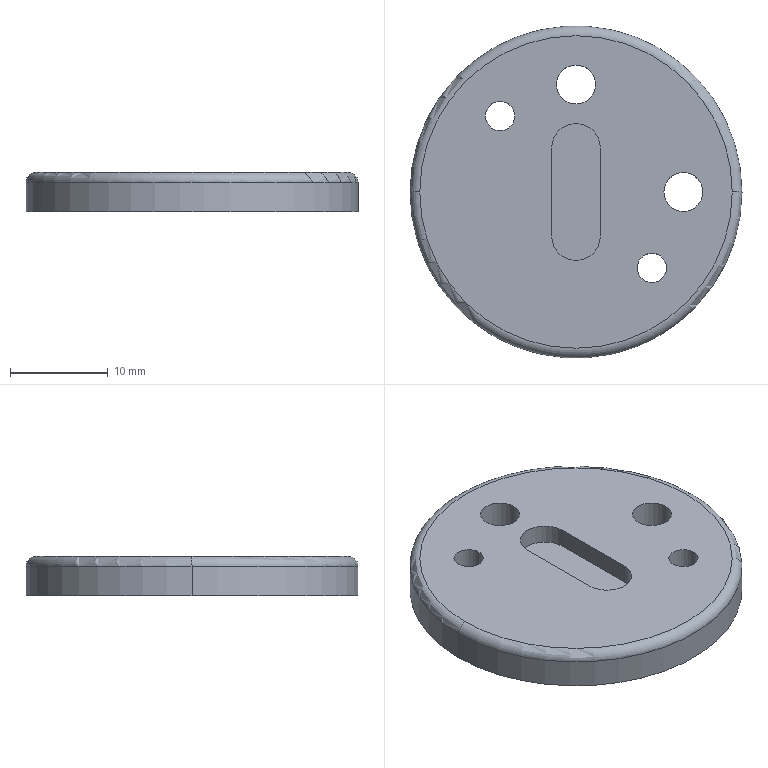Part | SolidWorks | features ICE 2, Extrusion 1, Fillet 1 | 1 solid | 19 faces | box 34 x 34 x 4 mm | volume 3323 mm3 | cylinder 12 | plane 5 | torus 2 | commonest cylinder face diameters 3 x4 4 x4 5 x2 34 x2
STEP:
#1=CARTESIAN_POINT('',(-17.,0.,3.));
#2=VERTEX_POINT('',#1);
#3=CARTESIAN_POINT('',(17.,0.,3.));
#4=VERTEX_POINT('',#3);
#5=CARTESIAN_POINT('',(0.,0.,3.));
#6=DIRECTION('',(0.,0.,-1.));
#7=DIRECTION('',(1.,0.,0.));
#8=AXIS2_PLACEMENT_3D('',#5,#6,#7);
#9=CIRCLE('',#8,17.);
#10=EDGE_CURVE('',#2,#4,#9,.T.);
#11=ORIENTED_EDGE('',*,*,#10,.F.);
#12=CARTESIAN_POINT('',(-16.,0.,4.));
#13=VERTEX_POINT('',#12);
#14=CARTESIAN_POINT('',(-16.,0.,3.));
#15=DIRECTION('',(0.,1.,0.));
#16=DIRECTION('',(-1.,0.,0.));
#17=AXIS2_PLACEMENT_3D('',#14,#15,#16);
#18=CIRCLE('',#17,1.);
#19=EDGE_CURVE('',#2,#13,#18,.T.);
#20=ORIENTED_EDGE('',*,*,#19,.T.);
#21=CARTESIAN_POINT('',(16.,0.,4.));
#22=VERTEX_POINT('',#21);
#23=CARTESIAN_POINT('',(0.,0.,4.));
#24=DIRECTION('',(0.,0.,1.));
#25=DIRECTION('',(1.,0.,0.));
#26=AXIS2_PLACEMENT_3D('',#23,#24,#25);
#27=CIRCLE('',#26,16.);
#28=EDGE_CURVE('',#22,#13,#27,.T.);
#29=ORIENTED_EDGE('',*,*,#28,.F.);
#30=CARTESIAN_POINT('',(16.,0.,3.));
#31=DIRECTION('',(0.,-1.,0.));
#32=DIRECTION('',(0.,0.,-1.));
#33=AXIS2_PLACEMENT_3D('',#30,#31,#32);
#34=CIRCLE('',#33,1.);
#35=EDGE_CURVE('',#4,#22,#34,.T.);
#36=ORIENTED_EDGE('',*,*,#35,.F.);
#37=EDGE_LOOP('',(#11,#20,#29,#36));
#38=FACE_OUTER_BOUND('',#37,.T.);
#39=CARTESIAN_POINT('',(0.,0.,3.));
#40=DIRECTION('',(0.,0.,1.));
#41=DIRECTION('',(1.,0.,0.));
#42=AXIS2_PLACEMENT_3D('',#39,#40,#41);
#43=TOROIDAL_SURFACE('',#42,16.,1.);
#44=ADVANCED_FACE('',(#38),#43,.T.);
#45=CARTESIAN_POINT('',(6.278,-7.778,0.));
#46=VERTEX_POINT('',#45);
#47=CARTESIAN_POINT('',(9.278,-7.778,0.));
#48=VERTEX_POINT('',#47);
#49=CARTESIAN_POINT('',(7.778,-7.778,0.));
#50=DIRECTION('',(0.,0.,1.));
#51=DIRECTION('',(1.,0.,0.));
#52=AXIS2_PLACEMENT_3D('',#49,#50,#51);
#53=CIRCLE('',#52,1.5);
#54=EDGE_CURVE('',#46,#48,#53,.T.);
#55=ORIENTED_EDGE('',*,*,#54,.F.);
#56=CARTESIAN_POINT('',(6.278,-7.778,4.));
#57=VERTEX_POINT('',#56);
#58=CARTESIAN_POINT('',(6.278,-7.778,0.));
#59=DIRECTION('',(0.,0.,1.));
#60=VECTOR('',#59,1000.);
#61=LINE('',#58,#60);
#62=EDGE_CURVE('',#46,#57,#61,.T.);
#63=ORIENTED_EDGE('',*,*,#62,.T.);
#64=CARTESIAN_POINT('',(9.278,-7.778,4.));
#65=VERTEX_POINT('',#64);
#66=CARTESIAN_POINT('',(7.778,-7.778,4.));
#67=DIRECTION('',(0.,0.,1.));
#68=DIRECTION('',(1.,0.,0.));
#69=AXIS2_PLACEMENT_3D('',#66,#67,#68);
#70=CIRCLE('',#69,1.5);
#71=EDGE_CURVE('',#57,#65,#70,.T.);
#72=ORIENTED_EDGE('',*,*,#71,.T.);
#73=CARTESIAN_POINT('',(9.278,-7.778,0.));
#74=DIRECTION('',(0.,0.,1.));
#75=VECTOR('',#74,1000.);
#76=LINE('',#73,#75);
#77=EDGE_CURVE('',#48,#65,#76,.T.);
#78=ORIENTED_EDGE('',*,*,#77,.F.);
#79=EDGE_LOOP('',(#55,#63,#72,#78));
#80=FACE_OUTER_BOUND('',#79,.T.);
#81=CARTESIAN_POINT('',(7.778,-7.778,0.));
#82=DIRECTION('',(0.,0.,1.));
#83=DIRECTION('',(1.,0.,0.));
#84=AXIS2_PLACEMENT_3D('',#81,#82,#83);
#85=CYLINDRICAL_SURFACE('',#84,1.5);
#86=ADVANCED_FACE('',(#80),#85,.F.);
#87=CARTESIAN_POINT('',(-9.278,7.778,0.));
#88=VERTEX_POINT('',#87);
#89=CARTESIAN_POINT('',(-6.278,7.778,0.));
#90=VERTEX_POINT('',#89);
#91=CARTESIAN_POINT('',(-7.778,7.778,0.));
#92=DIRECTION('',(0.,0.,1.));
#93=DIRECTION('',(1.,0.,0.));
#94=AXIS2_PLACEMENT_3D('',#91,#92,#93);
#95=CIRCLE('',#94,1.5);
#96=EDGE_CURVE('',#88,#90,#95,.T.);
#97=ORIENTED_EDGE('',*,*,#96,.F.);
#98=CARTESIAN_POINT('',(-9.278,7.778,4.));
#99=VERTEX_POINT('',#98);
#100=CARTESIAN_POINT('',(-9.278,7.778,0.));
#101=DIRECTION('',(0.,0.,1.));
#102=VECTOR('',#101,1000.);
#103=LINE('',#100,#102);
#104=EDGE_CURVE('',#88,#99,#103,.T.);
#105=ORIENTED_EDGE('',*,*,#104,.T.);
#106=CARTESIAN_POINT('',(-6.278,7.778,4.));
#107=VERTEX_POINT('',#106);
#108=CARTESIAN_POINT('',(-7.778,7.778,4.));
#109=DIRECTION('',(0.,0.,1.));
#110=DIRECTION('',(1.,0.,0.));
#111=AXIS2_PLACEMENT_3D('',#108,#109,#110);
#112=CIRCLE('',#111,1.5);
#113=EDGE_CURVE('',#99,#107,#112,.T.);
#114=ORIENTED_EDGE('',*,*,#113,.T.);
#115=CARTESIAN_POINT('',(-6.278,7.778,0.));
#116=DIRECTION('',(0.,0.,1.));
#117=VECTOR('',#116,1000.);
#118=LINE('',#115,#117);
#119=EDGE_CURVE('',#90,#107,#118,.T.);
#120=ORIENTED_EDGE('',*,*,#119,.F.);
#121=EDGE_LOOP('',(#97,#105,#114,#120));
#122=FACE_OUTER_BOUND('',#121,.T.);
#123=CARTESIAN_POINT('',(-7.778,7.778,0.));
#124=DIRECTION('',(0.,0.,1.));
#125=DIRECTION('',(1.,0.,0.));
#126=AXIS2_PLACEMENT_3D('',#123,#124,#125);
#127=CYLINDRICAL_SURFACE('',#126,1.5);
#128=ADVANCED_FACE('',(#122),#127,.F.);
#129=CARTESIAN_POINT('',(9.,0.,0.));
#130=VERTEX_POINT('',#129);
#131=CARTESIAN_POINT('',(13.,0.,0.));
#132=VERTEX_POINT('',#131);
#133=CARTESIAN_POINT('',(11.,0.,0.));
#134=DIRECTION('',(0.,0.,1.));
#135=DIRECTION('',(1.,0.,0.));
#136=AXIS2_PLACEMENT_3D('',#133,#134,#135);
#137=CIRCLE('',#136,2.);
#138=EDGE_CURVE('',#130,#132,#137,.T.);
#139=ORIENTED_EDGE('',*,*,#138,.F.);
#140=CARTESIAN_POINT('',(9.,0.,4.));
#141=VERTEX_POINT('',#140);
#142=CARTESIAN_POINT('',(9.,0.,0.));
#143=DIRECTION('',(0.,0.,1.));
#144=VECTOR('',#143,1000.);
#145=LINE('',#142,#144);
#146=EDGE_CURVE('',#130,#141,#145,.T.);
#147=ORIENTED_EDGE('',*,*,#146,.T.);
#148=CARTESIAN_POINT('',(13.,0.,4.));
#149=VERTEX_POINT('',#148);
#150=CARTESIAN_POINT('',(11.,0.,4.));
#151=DIRECTION('',(0.,0.,1.));
#152=DIRECTION('',(1.,0.,0.));
#153=AXIS2_PLACEMENT_3D('',#150,#151,#152);
#154=CIRCLE('',#153,2.);
#155=EDGE_CURVE('',#141,#149,#154,.T.);
#156=ORIENTED_EDGE('',*,*,#155,.T.);
#157=CARTESIAN_POINT('',(13.,0.,0.));
#158=DIRECTION('',(0.,0.,1.));
#159=VECTOR('',#158,1000.);
#160=LINE('',#157,#159);
#161=EDGE_CURVE('',#132,#149,#160,.T.);
#162=ORIENTED_EDGE('',*,*,#161,.F.);
#163=EDGE_LOOP('',(#139,#147,#156,#162));
#164=FACE_OUTER_BOUND('',#163,.T.);
#165=CARTESIAN_POINT('',(11.,0.,0.));
#166=DIRECTION('',(0.,0.,1.));
#167=DIRECTION('',(1.,0.,0.));
#168=AXIS2_PLACEMENT_3D('',#165,#166,#167);
#169=CYLINDRICAL_SURFACE('',#168,2.);
#170=ADVANCED_FACE('',(#164),#169,.F.);
#171=CARTESIAN_POINT('',(-2.,11.,0.));
#172=VERTEX_POINT('',#171);
#173=CARTESIAN_POINT('',(2.,11.,0.));
#174=VERTEX_POINT('',#173);
#175=CARTESIAN_POINT('',(0.,11.,0.));
#176=DIRECTION('',(0.,0.,1.));
#177=DIRECTION('',(1.,0.,0.));
#178=AXIS2_PLACEMENT_3D('',#175,#176,#177);
#179=CIRCLE('',#178,2.);
#180=EDGE_CURVE('',#172,#174,#179,.T.);
#181=ORIENTED_EDGE('',*,*,#180,.F.);
#182=CARTESIAN_POINT('',(-2.,11.,4.));
#183=VERTEX_POINT('',#182);
#184=CARTESIAN_POINT('',(-2.,11.,0.));
#185=DIRECTION('',(0.,0.,1.));
#186=VECTOR('',#185,1000.);
#187=LINE('',#184,#186);
#188=EDGE_CURVE('',#172,#183,#187,.T.);
#189=ORIENTED_EDGE('',*,*,#188,.T.);
#190=CARTESIAN_POINT('',(2.,11.,4.));
#191=VERTEX_POINT('',#190);
#192=CARTESIAN_POINT('',(0.,11.,4.));
#193=DIRECTION('',(0.,0.,1.));
#194=DIRECTION('',(1.,0.,0.));
#195=AXIS2_PLACEMENT_3D('',#192,#193,#194);
#196=CIRCLE('',#195,2.);
#197=EDGE_CURVE('',#183,#191,#196,.T.);
#198=ORIENTED_EDGE('',*,*,#197,.T.);
#199=CARTESIAN_POINT('',(2.,11.,0.));
#200=DIRECTION('',(0.,0.,1.));
#201=VECTOR('',#200,1000.);
#202=LINE('',#199,#201);
#203=EDGE_CURVE('',#174,#191,#202,.T.);
#204=ORIENTED_EDGE('',*,*,#203,.F.);
#205=EDGE_LOOP('',(#181,#189,#198,#204));
#206=FACE_OUTER_BOUND('',#205,.T.);
#207=CARTESIAN_POINT('',(0.,11.,0.));
#208=DIRECTION('',(0.,0.,1.));
#209=DIRECTION('',(1.,0.,0.));
#210=AXIS2_PLACEMENT_3D('',#207,#208,#209);
#211=CYLINDRICAL_SURFACE('',#210,2.);
#212=ADVANCED_FACE('',(#206),#211,.F.);
#213=ORIENTED_EDGE('',*,*,#10,.T.);
#214=CARTESIAN_POINT('',(17.,0.,0.));
#215=VERTEX_POINT('',#214);
#216=CARTESIAN_POINT('',(17.,0.,4.));
#217=DIRECTION('',(0.,0.,-1.));
#218=VECTOR('',#217,1000.);
#219=LINE('',#216,#218);
#220=EDGE_CURVE('',#4,#215,#219,.T.);
#221=ORIENTED_EDGE('',*,*,#220,.T.);
#222=CARTESIAN_POINT('',(-17.,0.,0.));
#223=VERTEX_POINT('',#222);
#224=CARTESIAN_POINT('',(0.,0.,0.));
#225=DIRECTION('',(0.,0.,1.));
#226=DIRECTION('',(1.,0.,0.));
#227=AXIS2_PLACEMENT_3D('',#224,#225,#226);
#228=CIRCLE('',#227,17.);
#229=EDGE_CURVE('',#215,#223,#228,.T.);
#230=ORIENTED_EDGE('',*,*,#229,.T.);
#231=CARTESIAN_POINT('',(-17.,0.,4.));
#232=DIRECTION('',(0.,0.,-1.));
#233=VECTOR('',#232,1000.);
#234=LINE('',#231,#233);
#235=EDGE_CURVE('',#2,#223,#234,.T.);
#236=ORIENTED_EDGE('',*,*,#235,.F.);
#237=EDGE_LOOP('',(#213,#221,#230,#236));
#238=FACE_OUTER_BOUND('',#237,.T.);
#239=CARTESIAN_POINT('',(0.,0.,4.));
#240=DIRECTION('',(0.,0.,-1.));
#241=DIRECTION('',(-1.,0.,0.));
#242=AXIS2_PLACEMENT_3D('',#239,#240,#241);
#243=CYLINDRICAL_SURFACE('',#242,17.);
#244=ADVANCED_FACE('',(#238),#243,.T.);
#245=ORIENTED_EDGE('',*,*,#220,.F.);
#246=CARTESIAN_POINT('',(0.,0.,3.));
#247=DIRECTION('',(0.,0.,-1.));
#248=DIRECTION('',(1.,0.,0.));
#249=AXIS2_PLACEMENT_3D('',#246,#247,#248);
#250=CIRCLE('',#249,17.);
#251=EDGE_CURVE('',#4,#2,#250,.T.);
#252=ORIENTED_EDGE('',*,*,#251,.T.);
#253=ORIENTED_EDGE('',*,*,#235,.T.);
#254=CARTESIAN_POINT('',(0.,0.,0.));
#255=DIRECTION('',(0.,0.,1.));
#256=DIRECTION('',(1.,0.,0.));
#257=AXIS2_PLACEMENT_3D('',#254,#255,#256);
#258=CIRCLE('',#257,17.);
#259=EDGE_CURVE('',#223,#215,#258,.T.);
#260=ORIENTED_EDGE('',*,*,#259,.T.);
#261=EDGE_LOOP('',(#245,#252,#253,#260));
#262=FACE_OUTER_BOUND('',#261,.T.);
#263=CARTESIAN_POINT('',(0.,0.,4.));
#264=DIRECTION('',(0.,0.,-1.));
#265=DIRECTION('',(-1.,0.,0.));
#266=AXIS2_PLACEMENT_3D('',#263,#264,#265);
#267=CYLINDRICAL_SURFACE('',#266,17.);
#268=ADVANCED_FACE('',(#262),#267,.T.);
#269=ORIENTED_EDGE('',*,*,#28,.T.);
#270=CARTESIAN_POINT('',(0.,0.,4.));
#271=DIRECTION('',(0.,0.,1.));
#272=DIRECTION('',(1.,0.,0.));
#273=AXIS2_PLACEMENT_3D('',#270,#271,#272);
#274=CIRCLE('',#273,16.);
#275=EDGE_CURVE('',#13,#22,#274,.T.);
#276=ORIENTED_EDGE('',*,*,#275,.T.);
#277=EDGE_LOOP('',(#269,#276));
#278=FACE_OUTER_BOUND('',#277,.T.);
#279=CARTESIAN_POINT('',(7.778,-7.778,4.));
#280=DIRECTION('',(0.,0.,1.));
#281=DIRECTION('',(1.,0.,0.));
#282=AXIS2_PLACEMENT_3D('',#279,#280,#281);
#283=CIRCLE('',#282,1.5);
#284=EDGE_CURVE('',#65,#57,#283,.T.);
#285=ORIENTED_EDGE('',*,*,#284,.F.);
#286=ORIENTED_EDGE('',*,*,#71,.F.);
#287=EDGE_LOOP('',(#285,#286));
#288=FACE_BOUND('',#287,.T.);
#289=CARTESIAN_POINT('',(-7.778,7.778,4.));
#290=DIRECTION('',(0.,0.,1.));
#291=DIRECTION('',(1.,0.,0.));
#292=AXIS2_PLACEMENT_3D('',#289,#290,#291);
#293=CIRCLE('',#292,1.5);
#294=EDGE_CURVE('',#107,#99,#293,.T.);
#295=ORIENTED_EDGE('',*,*,#294,.F.);
#296=ORIENTED_EDGE('',*,*,#113,.F.);
#297=EDGE_LOOP('',(#295,#296));
#298=FACE_BOUND('',#297,.T.);
#299=CARTESIAN_POINT('',(11.,0.,4.));
#300=DIRECTION('',(0.,0.,1.));
#301=DIRECTION('',(1.,0.,0.));
#302=AXIS2_PLACEMENT_3D('',#299,#300,#301);
#303=CIRCLE('',#302,2.);
#304=EDGE_CURVE('',#149,#141,#303,.T.);
#305=ORIENTED_EDGE('',*,*,#304,.F.);
#306=ORIENTED_EDGE('',*,*,#155,.F.);
#307=EDGE_LOOP('',(#305,#306));
#308=FACE_BOUND('',#307,.T.);
#309=CARTESIAN_POINT('',(0.,11.,4.));
#310=DIRECTION('',(0.,0.,1.));
#311=DIRECTION('',(1.,0.,0.));
#312=AXIS2_PLACEMENT_3D('',#309,#310,#311);
#313=CIRCLE('',#312,2.);
#314=EDGE_CURVE('',#191,#183,#313,.T.);
#315=ORIENTED_EDGE('',*,*,#314,.F.);
#316=ORIENTED_EDGE('',*,*,#197,.F.);
#317=EDGE_LOOP('',(#315,#316));
#318=FACE_BOUND('',#317,.T.);
#319=CARTESIAN_POINT('',(2.5,4.5,4.));
#320=VERTEX_POINT('',#319);
#321=CARTESIAN_POINT('',(-2.5,4.5,4.));
#322=VERTEX_POINT('',#321);
#323=CARTESIAN_POINT('',(0.,4.5,4.));
#324=DIRECTION('',(0.,0.,1.));
#325=DIRECTION('',(1.,0.,0.));
#326=AXIS2_PLACEMENT_3D('',#323,#324,#325);
#327=CIRCLE('',#326,2.5);
#328=EDGE_CURVE('',#320,#322,#327,.T.);
#329=ORIENTED_EDGE('',*,*,#328,.F.);
#330=CARTESIAN_POINT('',(2.5,-4.5,4.));
#331=VERTEX_POINT('',#330);
#332=CARTESIAN_POINT('',(2.5,4.5,4.));
#333=DIRECTION('',(0.,1.,0.));
#334=VECTOR('',#333,1000.);
#335=LINE('',#332,#334);
#336=EDGE_CURVE('',#331,#320,#335,.T.);
#337=ORIENTED_EDGE('',*,*,#336,.F.);
#338=CARTESIAN_POINT('',(-2.5,-4.5,4.));
#339=VERTEX_POINT('',#338);
#340=CARTESIAN_POINT('',(0.,-4.5,4.));
#341=DIRECTION('',(0.,0.,1.));
#342=DIRECTION('',(1.,0.,0.));
#343=AXIS2_PLACEMENT_3D('',#340,#341,#342);
#344=CIRCLE('',#343,2.5);
#345=EDGE_CURVE('',#339,#331,#344,.T.);
#346=ORIENTED_EDGE('',*,*,#345,.F.);
#347=CARTESIAN_POINT('',(-2.5,4.5,4.));
#348=DIRECTION('',(0.,-1.,0.));
#349=VECTOR('',#348,1000.);
#350=LINE('',#347,#349);
#351=EDGE_CURVE('',#322,#339,#350,.T.);
#352=ORIENTED_EDGE('',*,*,#351,.F.);
#353=EDGE_LOOP('',(#329,#337,#346,#352));
#354=FACE_BOUND('',#353,.T.);
#355=CARTESIAN_POINT('',(0.,0.,4.));
#356=DIRECTION('',(0.,0.,1.));
#357=DIRECTION('',(1.,0.,0.));
#358=AXIS2_PLACEMENT_3D('',#355,#356,#357);
#359=PLANE('',#358);
#360=ADVANCED_FACE('',(#278,#288,#298,#308,#318,#354),#359,.T.);
#361=CARTESIAN_POINT('',(7.778,-7.778,0.));
#362=DIRECTION('',(0.,0.,1.));
#363=DIRECTION('',(1.,0.,0.));
#364=AXIS2_PLACEMENT_3D('',#361,#362,#363);
#365=CIRCLE('',#364,1.5);
#366=EDGE_CURVE('',#48,#46,#365,.T.);
#367=ORIENTED_EDGE('',*,*,#366,.T.);
#368=ORIENTED_EDGE('',*,*,#54,.T.);
#369=EDGE_LOOP('',(#367,#368));
#370=FACE_BOUND('',#369,.T.);
#371=CARTESIAN_POINT('',(-7.778,7.778,0.));
#372=DIRECTION('',(0.,0.,1.));
#373=DIRECTION('',(1.,0.,0.));
#374=AXIS2_PLACEMENT_3D('',#371,#372,#373);
#375=CIRCLE('',#374,1.5);
#376=EDGE_CURVE('',#90,#88,#375,.T.);
#377=ORIENTED_EDGE('',*,*,#376,.T.);
#378=ORIENTED_EDGE('',*,*,#96,.T.);
#379=EDGE_LOOP('',(#377,#378));
#380=FACE_BOUND('',#379,.T.);
#381=CARTESIAN_POINT('',(11.,0.,0.));
#382=DIRECTION('',(0.,0.,1.));
#383=DIRECTION('',(1.,0.,0.));
#384=AXIS2_PLACEMENT_3D('',#381,#382,#383);
#385=CIRCLE('',#384,2.);
#386=EDGE_CURVE('',#132,#130,#385,.T.);
#387=ORIENTED_EDGE('',*,*,#386,.T.);
#388=ORIENTED_EDGE('',*,*,#138,.T.);
#389=EDGE_LOOP('',(#387,#388));
#390=FACE_BOUND('',#389,.T.);
#391=CARTESIAN_POINT('',(0.,11.,0.));
#392=DIRECTION('',(0.,0.,1.));
#393=DIRECTION('',(1.,0.,0.));
#394=AXIS2_PLACEMENT_3D('',#391,#392,#393);
#395=CIRCLE('',#394,2.);
#396=EDGE_CURVE('',#174,#172,#395,.T.);
#397=ORIENTED_EDGE('',*,*,#396,.T.);
#398=ORIENTED_EDGE('',*,*,#180,.T.);
#399=EDGE_LOOP('',(#397,#398));
#400=FACE_BOUND('',#399,.T.);
#401=ORIENTED_EDGE('',*,*,#259,.F.);
#402=ORIENTED_EDGE('',*,*,#229,.F.);
#403=EDGE_LOOP('',(#401,#402));
#404=FACE_OUTER_BOUND('',#403,.T.);
#405=CARTESIAN_POINT('',(0.,0.,0.));
#406=DIRECTION('',(0.,0.,1.));
#407=DIRECTION('',(1.,0.,0.));
#408=AXIS2_PLACEMENT_3D('',#405,#406,#407);
#409=PLANE('',#408);
#410=ADVANCED_FACE('',(#370,#380,#390,#400,#404),#409,.F.);
#411=ORIENTED_EDGE('',*,*,#328,.T.);
#412=CARTESIAN_POINT('',(-2.5,4.5,2.));
#413=VERTEX_POINT('',#412);
#414=CARTESIAN_POINT('',(-2.5,4.5,2.));
#415=DIRECTION('',(0.,0.,1.));
#416=VECTOR('',#415,1000.);
#417=LINE('',#414,#416);
#418=EDGE_CURVE('',#413,#322,#417,.T.);
#419=ORIENTED_EDGE('',*,*,#418,.F.);
#420=CARTESIAN_POINT('',(2.5,4.5,2.));
#421=VERTEX_POINT('',#420);
#422=CARTESIAN_POINT('',(0.,4.5,2.));
#423=DIRECTION('',(0.,0.,1.));
#424=DIRECTION('',(1.,0.,0.));
#425=AXIS2_PLACEMENT_3D('',#422,#423,#424);
#426=CIRCLE('',#425,2.5);
#427=EDGE_CURVE('',#421,#413,#426,.T.);
#428=ORIENTED_EDGE('',*,*,#427,.F.);
#429=CARTESIAN_POINT('',(2.5,4.5,2.));
#430=DIRECTION('',(0.,0.,1.));
#431=VECTOR('',#430,1000.);
#432=LINE('',#429,#431);
#433=EDGE_CURVE('',#421,#320,#432,.T.);
#434=ORIENTED_EDGE('',*,*,#433,.T.);
#435=EDGE_LOOP('',(#411,#419,#428,#434));
#436=FACE_OUTER_BOUND('',#435,.T.);
#437=CARTESIAN_POINT('',(0.,4.5,2.));
#438=DIRECTION('',(0.,0.,1.));
#439=DIRECTION('',(1.,0.,0.));
#440=AXIS2_PLACEMENT_3D('',#437,#438,#439);
#441=CYLINDRICAL_SURFACE('',#440,2.5);
#442=ADVANCED_FACE('',(#436),#441,.F.);
#443=ORIENTED_EDGE('',*,*,#336,.T.);
#444=ORIENTED_EDGE('',*,*,#433,.F.);
#445=CARTESIAN_POINT('',(2.5,-4.5,2.));
#446=VERTEX_POINT('',#445);
#447=CARTESIAN_POINT('',(2.5,4.5,2.));
#448=DIRECTION('',(0.,1.,0.));
#449=VECTOR('',#448,1000.);
#450=LINE('',#447,#449);
#451=EDGE_CURVE('',#446,#421,#450,.T.);
#452=ORIENTED_EDGE('',*,*,#451,.F.);
#453=CARTESIAN_POINT('',(2.5,-4.5,2.));
#454=DIRECTION('',(0.,0.,1.));
#455=VECTOR('',#454,1000.);
#456=LINE('',#453,#455);
#457=EDGE_CURVE('',#446,#331,#456,.T.);
#458=ORIENTED_EDGE('',*,*,#457,.T.);
#459=EDGE_LOOP('',(#443,#444,#452,#458));
#460=FACE_OUTER_BOUND('',#459,.T.);
#461=CARTESIAN_POINT('',(2.5,4.5,2.));
#462=DIRECTION('',(1.,0.,0.));
#463=DIRECTION('',(0.,0.,-1.));
#464=AXIS2_PLACEMENT_3D('',#461,#462,#463);
#465=PLANE('',#464);
#466=ADVANCED_FACE('',(#460),#465,.F.);
#467=ORIENTED_EDGE('',*,*,#345,.T.);
#468=ORIENTED_EDGE('',*,*,#457,.F.);
#469=CARTESIAN_POINT('',(-2.5,-4.5,2.));
#470=VERTEX_POINT('',#469);
#471=CARTESIAN_POINT('',(0.,-4.5,2.));
#472=DIRECTION('',(0.,0.,1.));
#473=DIRECTION('',(1.,0.,0.));
#474=AXIS2_PLACEMENT_3D('',#471,#472,#473);
#475=CIRCLE('',#474,2.5);
#476=EDGE_CURVE('',#470,#446,#475,.T.);
#477=ORIENTED_EDGE('',*,*,#476,.F.);
#478=CARTESIAN_POINT('',(-2.5,-4.5,2.));
#479=DIRECTION('',(0.,0.,1.));
#480=VECTOR('',#479,1000.);
#481=LINE('',#478,#480);
#482=EDGE_CURVE('',#470,#339,#481,.T.);
#483=ORIENTED_EDGE('',*,*,#482,.T.);
#484=EDGE_LOOP('',(#467,#468,#477,#483));
#485=FACE_OUTER_BOUND('',#484,.T.);
#486=CARTESIAN_POINT('',(0.,-4.5,2.));
#487=DIRECTION('',(0.,0.,1.));
#488=DIRECTION('',(1.,0.,0.));
#489=AXIS2_PLACEMENT_3D('',#486,#487,#488);
#490=CYLINDRICAL_SURFACE('',#489,2.5);
#491=ADVANCED_FACE('',(#485),#490,.F.);
#492=ORIENTED_EDGE('',*,*,#351,.T.);
#493=ORIENTED_EDGE('',*,*,#482,.F.);
#494=CARTESIAN_POINT('',(-2.5,4.5,2.));
#495=DIRECTION('',(0.,-1.,0.));
#496=VECTOR('',#495,1000.);
#497=LINE('',#494,#496);
#498=EDGE_CURVE('',#413,#470,#497,.T.);
#499=ORIENTED_EDGE('',*,*,#498,.F.);
#500=ORIENTED_EDGE('',*,*,#418,.T.);
#501=EDGE_LOOP('',(#492,#493,#499,#500));
#502=FACE_OUTER_BOUND('',#501,.T.);
#503=CARTESIAN_POINT('',(-2.5,4.5,2.));
#504=DIRECTION('',(-1.,0.,0.));
#505=DIRECTION('',(0.,0.,1.));
#506=AXIS2_PLACEMENT_3D('',#503,#504,#505);
#507=PLANE('',#506);
#508=ADVANCED_FACE('',(#502),#507,.F.);
#509=ORIENTED_EDGE('',*,*,#427,.T.);
#510=ORIENTED_EDGE('',*,*,#498,.T.);
#511=ORIENTED_EDGE('',*,*,#476,.T.);
#512=ORIENTED_EDGE('',*,*,#451,.T.);
#513=EDGE_LOOP('',(#509,#510,#511,#512));
#514=FACE_OUTER_BOUND('',#513,.T.);
#515=CARTESIAN_POINT('',(0.,4.5,2.));
#516=DIRECTION('',(0.,0.,1.));
#517=DIRECTION('',(1.,0.,0.));
#518=AXIS2_PLACEMENT_3D('',#515,#516,#517);
#519=PLANE('',#518);
#520=ADVANCED_FACE('',(#514),#519,.T.);
#521=ORIENTED_EDGE('',*,*,#188,.F.);
#522=ORIENTED_EDGE('',*,*,#396,.F.);
#523=ORIENTED_EDGE('',*,*,#203,.T.);
#524=ORIENTED_EDGE('',*,*,#314,.T.);
#525=EDGE_LOOP('',(#521,#522,#523,#524));
#526=FACE_OUTER_BOUND('',#525,.T.);
#527=CARTESIAN_POINT('',(0.,11.,0.));
#528=DIRECTION('',(0.,0.,1.));
#529=DIRECTION('',(1.,0.,0.));
#530=AXIS2_PLACEMENT_3D('',#527,#528,#529);
#531=CYLINDRICAL_SURFACE('',#530,2.);
#532=ADVANCED_FACE('',(#526),#531,.F.);
#533=ORIENTED_EDGE('',*,*,#146,.F.);
#534=ORIENTED_EDGE('',*,*,#386,.F.);
#535=ORIENTED_EDGE('',*,*,#161,.T.);
#536=ORIENTED_EDGE('',*,*,#304,.T.);
#537=EDGE_LOOP('',(#533,#534,#535,#536));
#538=FACE_OUTER_BOUND('',#537,.T.);
#539=CARTESIAN_POINT('',(11.,0.,0.));
#540=DIRECTION('',(0.,0.,1.));
#541=DIRECTION('',(1.,0.,0.));
#542=AXIS2_PLACEMENT_3D('',#539,#540,#541);
#543=CYLINDRICAL_SURFACE('',#542,2.);
#544=ADVANCED_FACE('',(#538),#543,.F.);
#545=ORIENTED_EDGE('',*,*,#104,.F.);
#546=ORIENTED_EDGE('',*,*,#376,.F.);
#547=ORIENTED_EDGE('',*,*,#119,.T.);
#548=ORIENTED_EDGE('',*,*,#294,.T.);
#549=EDGE_LOOP('',(#545,#546,#547,#548));
#550=FACE_OUTER_BOUND('',#549,.T.);
#551=CARTESIAN_POINT('',(-7.778,7.778,0.));
#552=DIRECTION('',(0.,0.,1.));
#553=DIRECTION('',(1.,0.,0.));
#554=AXIS2_PLACEMENT_3D('',#551,#552,#553);
#555=CYLINDRICAL_SURFACE('',#554,1.5);
#556=ADVANCED_FACE('',(#550),#555,.F.);
#557=ORIENTED_EDGE('',*,*,#62,.F.);
#558=ORIENTED_EDGE('',*,*,#366,.F.);
#559=ORIENTED_EDGE('',*,*,#77,.T.);
#560=ORIENTED_EDGE('',*,*,#284,.T.);
#561=EDGE_LOOP('',(#557,#558,#559,#560));
#562=FACE_OUTER_BOUND('',#561,.T.);
#563=CARTESIAN_POINT('',(7.778,-7.778,0.));
#564=DIRECTION('',(0.,0.,1.));
#565=DIRECTION('',(1.,0.,0.));
#566=AXIS2_PLACEMENT_3D('',#563,#564,#565);
#567=CYLINDRICAL_SURFACE('',#566,1.5);
#568=ADVANCED_FACE('',(#562),#567,.F.);
#569=ORIENTED_EDGE('',*,*,#19,.F.);
#570=ORIENTED_EDGE('',*,*,#251,.F.);
#571=ORIENTED_EDGE('',*,*,#35,.T.);
#572=ORIENTED_EDGE('',*,*,#275,.F.);
#573=EDGE_LOOP('',(#569,#570,#571,#572));
#574=FACE_OUTER_BOUND('',#573,.T.);
#575=CARTESIAN_POINT('',(0.,0.,3.));
#576=DIRECTION('',(0.,0.,1.));
#577=DIRECTION('',(1.,0.,0.));
#578=AXIS2_PLACEMENT_3D('',#575,#576,#577);
#579=TOROIDAL_SURFACE('',#578,16.,1.);
#580=ADVANCED_FACE('',(#574),#579,.T.);
#581=CLOSED_SHELL('',(#44,#86,#128,#170,#212,#244,#268,#360,#410,#442,#466,#491,#508,#520,#532,#544,#556,#568,#580));
#582=MANIFOLD_SOLID_BREP('',#581);
#583=CARTESIAN_POINT('',(0.,0.,0.));
#584=DIRECTION('',(0.,0.,1.));
#585=DIRECTION('',(1.,0.,0.));
#586=AXIS2_PLACEMENT_3D('',#583,#584,#585);
#587=(LENGTH_UNIT()NAMED_UNIT(*)SI_UNIT(.MILLI.,.METRE.));
#588=UNCERTAINTY_MEASURE_WITH_UNIT(LENGTH_MEASURE(0.00001),#587,'','');
#589=(NAMED_UNIT(*)PLANE_ANGLE_UNIT()SI_UNIT($,.RADIAN.));
#590=(NAMED_UNIT(*)SI_UNIT($,.STERADIAN.)SOLID_ANGLE_UNIT());
#591=(GEOMETRIC_REPRESENTATION_CONTEXT(3)GLOBAL_UNCERTAINTY_ASSIGNED_CONTEXT((#588))GLOBAL_UNIT_ASSIGNED_CONTEXT((#587,#589,#590))REPRESENTATION_CONTEXT('',''));
#592=ADVANCED_BREP_SHAPE_REPRESENTATION('',(#582,#586),#591);